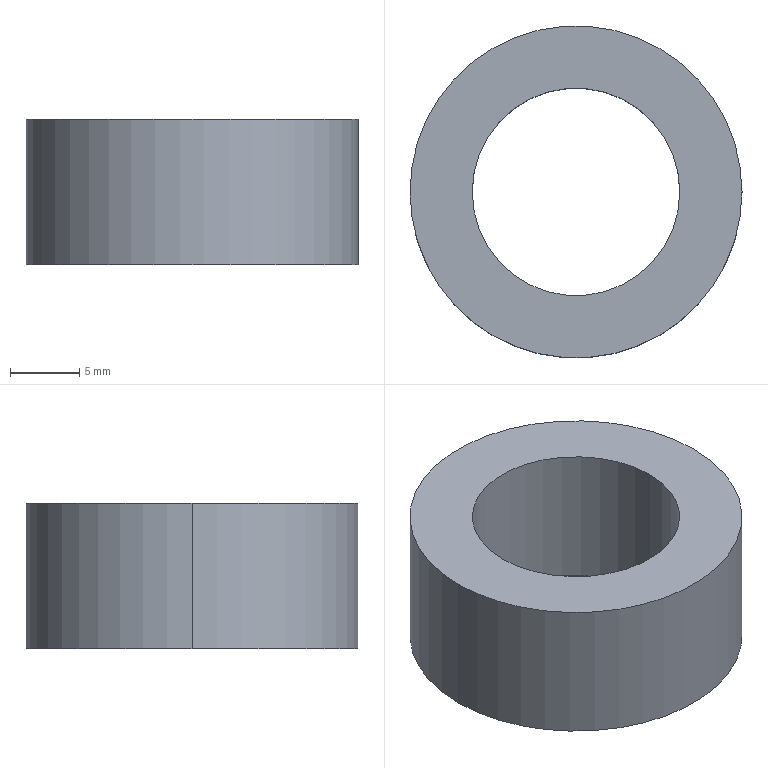Part | STEP file | PN_0019 (stop plate) | 1 solid | 6 faces | box 24 x 24 x 10.5 mm | volume 2895 mm3 | cylinder 4 | plane 2 | commonest cylinder face diameters 15 x2 24 x2
STEP:
#1=CARTESIAN_POINT('',(0.,0.,0.));
#2=DIRECTION('',(0.,0.,1.));
#3=DIRECTION('',(1.,0.,0.));
#4=AXIS2_PLACEMENT_3D('',#1,#2,#3);
#5=CARTESIAN_POINT('',(-7.5,0.,10.5));
#6=VERTEX_POINT('',#5);
#7=CARTESIAN_POINT('',(-7.5,0.,0.));
#8=VERTEX_POINT('',#7);
#9=CARTESIAN_POINT('',(-7.5,0.,10.5));
#10=DIRECTION('',(0.,0.,-1.));
#11=VECTOR('',#10,1.);
#12=LINE('',#9,#11);
#13=CARTESIAN_POINT('',(0.,0.,10.5));
#14=DIRECTION('',(0.,0.,-1.));
#15=DIRECTION('',(-1.,0.,0.));
#16=AXIS2_PLACEMENT_3D('',#13,#14,#15);
#17=CYLINDRICAL_SURFACE('',#16,7.5);
#18=CARTESIAN_POINT('',(6.283,0.));
#19=DIRECTION('',(0.,1.));
#20=VECTOR('',#19,1.);
#21=LINE('',#18,#20);
#22=(GEOMETRIC_REPRESENTATION_CONTEXT(2)PARAMETRIC_REPRESENTATION_CONTEXT()REPRESENTATION_CONTEXT('',''));
#23=DEFINITIONAL_REPRESENTATION('',(#21),#22);
#24=PCURVE('',#17,#23);
#25=CARTESIAN_POINT('',(0.,0.,10.5));
#26=DIRECTION('',(0.,0.,-1.));
#27=DIRECTION('',(-1.,0.,0.));
#28=AXIS2_PLACEMENT_3D('',#25,#26,#27);
#29=CYLINDRICAL_SURFACE('',#28,7.5);
#30=CARTESIAN_POINT('',(0.,0.));
#31=DIRECTION('',(0.,1.));
#32=VECTOR('',#31,1.);
#33=LINE('',#30,#32);
#34=(GEOMETRIC_REPRESENTATION_CONTEXT(2)PARAMETRIC_REPRESENTATION_CONTEXT()REPRESENTATION_CONTEXT('',''));
#35=DEFINITIONAL_REPRESENTATION('',(#33),#34);
#36=PCURVE('',#29,#35);
#37=SURFACE_CURVE('',#12,(#24,#36),.PCURVE_S1.);
#38=EDGE_CURVE('',#6,#8,#37,.T.);
#39=ORIENTED_EDGE('',*,*,#38,.T.);
#40=CARTESIAN_POINT('',(7.5,0.,0.));
#41=VERTEX_POINT('',#40);
#42=CARTESIAN_POINT('',(0.,0.,0.));
#43=DIRECTION('',(0.,0.,1.));
#44=DIRECTION('',(1.,0.,0.));
#45=AXIS2_PLACEMENT_3D('',#42,#43,#44);
#46=CIRCLE('',#45,7.5);
#47=CARTESIAN_POINT('',(9.425,10.5));
#48=DIRECTION('',(-1.,0.));
#49=VECTOR('',#48,1.);
#50=LINE('',#47,#49);
#51=(GEOMETRIC_REPRESENTATION_CONTEXT(2)PARAMETRIC_REPRESENTATION_CONTEXT()REPRESENTATION_CONTEXT('',''));
#52=DEFINITIONAL_REPRESENTATION('',(#50),#51);
#53=PCURVE('',#17,#52);
#54=CARTESIAN_POINT('',(0.,0.,0.));
#55=DIRECTION('',(0.,0.,1.));
#56=DIRECTION('',(1.,0.,0.));
#57=AXIS2_PLACEMENT_3D('',#54,#55,#56);
#58=PLANE('',#57);
#59=CARTESIAN_POINT('',(0.,0.));
#60=DIRECTION('',(1.,0.));
#61=AXIS2_PLACEMENT_2D('',#59,#60);
#62=CIRCLE('',#61,7.5);
#63=(GEOMETRIC_REPRESENTATION_CONTEXT(2)PARAMETRIC_REPRESENTATION_CONTEXT()REPRESENTATION_CONTEXT('',''));
#64=DEFINITIONAL_REPRESENTATION('',(#62),#63);
#65=PCURVE('',#58,#64);
#66=SURFACE_CURVE('',#46,(#53,#65),.PCURVE_S1.);
#67=EDGE_CURVE('',#8,#41,#66,.T.);
#68=ORIENTED_EDGE('',*,*,#67,.T.);
#69=CARTESIAN_POINT('',(7.5,0.,10.5));
#70=VERTEX_POINT('',#69);
#71=CARTESIAN_POINT('',(7.5,0.,10.5));
#72=DIRECTION('',(0.,0.,-1.));
#73=VECTOR('',#72,1.);
#74=LINE('',#71,#73);
#75=CARTESIAN_POINT('',(3.142,0.));
#76=DIRECTION('',(0.,1.));
#77=VECTOR('',#76,1.);
#78=LINE('',#75,#77);
#79=(GEOMETRIC_REPRESENTATION_CONTEXT(2)PARAMETRIC_REPRESENTATION_CONTEXT()REPRESENTATION_CONTEXT('',''));
#80=DEFINITIONAL_REPRESENTATION('',(#78),#79);
#81=PCURVE('',#17,#80);
#82=CARTESIAN_POINT('',(3.142,0.));
#83=DIRECTION('',(0.,1.));
#84=VECTOR('',#83,1.);
#85=LINE('',#82,#84);
#86=(GEOMETRIC_REPRESENTATION_CONTEXT(2)PARAMETRIC_REPRESENTATION_CONTEXT()REPRESENTATION_CONTEXT('',''));
#87=DEFINITIONAL_REPRESENTATION('',(#85),#86);
#88=PCURVE('',#29,#87);
#89=SURFACE_CURVE('',#74,(#81,#88),.PCURVE_S1.);
#90=EDGE_CURVE('',#70,#41,#89,.T.);
#91=ORIENTED_EDGE('',*,*,#90,.F.);
#92=CARTESIAN_POINT('',(0.,0.,10.5));
#93=DIRECTION('',(0.,0.,1.));
#94=DIRECTION('',(1.,0.,0.));
#95=AXIS2_PLACEMENT_3D('',#92,#93,#94);
#96=CIRCLE('',#95,7.5);
#97=CARTESIAN_POINT('',(9.425,0.));
#98=DIRECTION('',(-1.,0.));
#99=VECTOR('',#98,1.);
#100=LINE('',#97,#99);
#101=(GEOMETRIC_REPRESENTATION_CONTEXT(2)PARAMETRIC_REPRESENTATION_CONTEXT()REPRESENTATION_CONTEXT('',''));
#102=DEFINITIONAL_REPRESENTATION('',(#100),#101);
#103=PCURVE('',#17,#102);
#104=CARTESIAN_POINT('',(0.,0.,10.5));
#105=DIRECTION('',(0.,0.,1.));
#106=DIRECTION('',(1.,0.,0.));
#107=AXIS2_PLACEMENT_3D('',#104,#105,#106);
#108=PLANE('',#107);
#109=CARTESIAN_POINT('',(0.,0.));
#110=DIRECTION('',(1.,0.));
#111=AXIS2_PLACEMENT_2D('',#109,#110);
#112=CIRCLE('',#111,7.5);
#113=(GEOMETRIC_REPRESENTATION_CONTEXT(2)PARAMETRIC_REPRESENTATION_CONTEXT()REPRESENTATION_CONTEXT('',''));
#114=DEFINITIONAL_REPRESENTATION('',(#112),#113);
#115=PCURVE('',#108,#114);
#116=SURFACE_CURVE('',#96,(#103,#115),.PCURVE_S1.);
#117=EDGE_CURVE('',#6,#70,#116,.T.);
#118=ORIENTED_EDGE('',*,*,#117,.F.);
#119=EDGE_LOOP('',(#39,#68,#91,#118));
#120=FACE_BOUND('',#119,.F.);
#121=ADVANCED_FACE('',(#120),#17,.F.);
#122=CARTESIAN_POINT('',(12.,0.,10.5));
#123=VERTEX_POINT('',#122);
#124=CARTESIAN_POINT('',(-12.,0.,10.5));
#125=VERTEX_POINT('',#124);
#126=CARTESIAN_POINT('',(0.,0.,10.5));
#127=DIRECTION('',(0.,0.,1.));
#128=DIRECTION('',(1.,0.,0.));
#129=AXIS2_PLACEMENT_3D('',#126,#127,#128);
#130=CIRCLE('',#129,12.);
#131=CARTESIAN_POINT('',(0.,0.,10.5));
#132=DIRECTION('',(0.,0.,-1.));
#133=DIRECTION('',(-1.,0.,0.));
#134=AXIS2_PLACEMENT_3D('',#131,#132,#133);
#135=CYLINDRICAL_SURFACE('',#134,12.);
#136=CARTESIAN_POINT('',(3.142,0.));
#137=DIRECTION('',(-1.,0.));
#138=VECTOR('',#137,1.);
#139=LINE('',#136,#138);
#140=(GEOMETRIC_REPRESENTATION_CONTEXT(2)PARAMETRIC_REPRESENTATION_CONTEXT()REPRESENTATION_CONTEXT('',''));
#141=DEFINITIONAL_REPRESENTATION('',(#139),#140);
#142=PCURVE('',#135,#141);
#143=CARTESIAN_POINT('',(0.,0.));
#144=DIRECTION('',(1.,0.));
#145=AXIS2_PLACEMENT_2D('',#143,#144);
#146=CIRCLE('',#145,12.);
#147=(GEOMETRIC_REPRESENTATION_CONTEXT(2)PARAMETRIC_REPRESENTATION_CONTEXT()REPRESENTATION_CONTEXT('',''));
#148=DEFINITIONAL_REPRESENTATION('',(#146),#147);
#149=PCURVE('',#108,#148);
#150=SURFACE_CURVE('',#130,(#142,#149),.PCURVE_S1.);
#151=EDGE_CURVE('',#123,#125,#150,.T.);
#152=ORIENTED_EDGE('',*,*,#151,.F.);
#153=CARTESIAN_POINT('',(12.,0.,0.));
#154=VERTEX_POINT('',#153);
#155=CARTESIAN_POINT('',(12.,0.,10.5));
#156=DIRECTION('',(0.,0.,-1.));
#157=VECTOR('',#156,1.);
#158=LINE('',#155,#157);
#159=CARTESIAN_POINT('',(3.142,0.));
#160=DIRECTION('',(0.,1.));
#161=VECTOR('',#160,1.);
#162=LINE('',#159,#161);
#163=(GEOMETRIC_REPRESENTATION_CONTEXT(2)PARAMETRIC_REPRESENTATION_CONTEXT()REPRESENTATION_CONTEXT('',''));
#164=DEFINITIONAL_REPRESENTATION('',(#162),#163);
#165=PCURVE('',#135,#164);
#166=CARTESIAN_POINT('',(0.,0.,10.5));
#167=DIRECTION('',(0.,0.,-1.));
#168=DIRECTION('',(-1.,0.,0.));
#169=AXIS2_PLACEMENT_3D('',#166,#167,#168);
#170=CYLINDRICAL_SURFACE('',#169,12.);
#171=CARTESIAN_POINT('',(3.142,0.));
#172=DIRECTION('',(0.,1.));
#173=VECTOR('',#172,1.);
#174=LINE('',#171,#173);
#175=(GEOMETRIC_REPRESENTATION_CONTEXT(2)PARAMETRIC_REPRESENTATION_CONTEXT()REPRESENTATION_CONTEXT('',''));
#176=DEFINITIONAL_REPRESENTATION('',(#174),#175);
#177=PCURVE('',#170,#176);
#178=SURFACE_CURVE('',#158,(#165,#177),.PCURVE_S1.);
#179=EDGE_CURVE('',#123,#154,#178,.T.);
#180=ORIENTED_EDGE('',*,*,#179,.T.);
#181=CARTESIAN_POINT('',(-12.,0.,0.));
#182=VERTEX_POINT('',#181);
#183=CARTESIAN_POINT('',(0.,0.,0.));
#184=DIRECTION('',(0.,0.,1.));
#185=DIRECTION('',(1.,0.,0.));
#186=AXIS2_PLACEMENT_3D('',#183,#184,#185);
#187=CIRCLE('',#186,12.);
#188=CARTESIAN_POINT('',(3.142,10.5));
#189=DIRECTION('',(-1.,0.));
#190=VECTOR('',#189,1.);
#191=LINE('',#188,#190);
#192=(GEOMETRIC_REPRESENTATION_CONTEXT(2)PARAMETRIC_REPRESENTATION_CONTEXT()REPRESENTATION_CONTEXT('',''));
#193=DEFINITIONAL_REPRESENTATION('',(#191),#192);
#194=PCURVE('',#135,#193);
#195=CARTESIAN_POINT('',(0.,0.));
#196=DIRECTION('',(1.,0.));
#197=AXIS2_PLACEMENT_2D('',#195,#196);
#198=CIRCLE('',#197,12.);
#199=(GEOMETRIC_REPRESENTATION_CONTEXT(2)PARAMETRIC_REPRESENTATION_CONTEXT()REPRESENTATION_CONTEXT('',''));
#200=DEFINITIONAL_REPRESENTATION('',(#198),#199);
#201=PCURVE('',#58,#200);
#202=SURFACE_CURVE('',#187,(#194,#201),.PCURVE_S1.);
#203=EDGE_CURVE('',#154,#182,#202,.T.);
#204=ORIENTED_EDGE('',*,*,#203,.T.);
#205=CARTESIAN_POINT('',(-12.,0.,10.5));
#206=DIRECTION('',(0.,0.,-1.));
#207=VECTOR('',#206,1.);
#208=LINE('',#205,#207);
#209=CARTESIAN_POINT('',(0.,0.));
#210=DIRECTION('',(0.,1.));
#211=VECTOR('',#210,1.);
#212=LINE('',#209,#211);
#213=(GEOMETRIC_REPRESENTATION_CONTEXT(2)PARAMETRIC_REPRESENTATION_CONTEXT()REPRESENTATION_CONTEXT('',''));
#214=DEFINITIONAL_REPRESENTATION('',(#212),#213);
#215=PCURVE('',#135,#214);
#216=CARTESIAN_POINT('',(6.283,0.));
#217=DIRECTION('',(0.,1.));
#218=VECTOR('',#217,1.);
#219=LINE('',#216,#218);
#220=(GEOMETRIC_REPRESENTATION_CONTEXT(2)PARAMETRIC_REPRESENTATION_CONTEXT()REPRESENTATION_CONTEXT('',''));
#221=DEFINITIONAL_REPRESENTATION('',(#219),#220);
#222=PCURVE('',#170,#221);
#223=SURFACE_CURVE('',#208,(#215,#222),.PCURVE_S1.);
#224=EDGE_CURVE('',#125,#182,#223,.T.);
#225=ORIENTED_EDGE('',*,*,#224,.F.);
#226=EDGE_LOOP('',(#152,#180,#204,#225));
#227=FACE_BOUND('',#226,.T.);
#228=ADVANCED_FACE('',(#227),#135,.T.);
#229=CARTESIAN_POINT('',(0.,0.,10.5));
#230=DIRECTION('',(0.,0.,1.));
#231=DIRECTION('',(1.,0.,0.));
#232=AXIS2_PLACEMENT_3D('',#229,#230,#231);
#233=CIRCLE('',#232,12.);
#234=CARTESIAN_POINT('',(0.,0.));
#235=DIRECTION('',(1.,0.));
#236=AXIS2_PLACEMENT_2D('',#234,#235);
#237=CIRCLE('',#236,12.);
#238=(GEOMETRIC_REPRESENTATION_CONTEXT(2)PARAMETRIC_REPRESENTATION_CONTEXT()REPRESENTATION_CONTEXT('',''));
#239=DEFINITIONAL_REPRESENTATION('',(#237),#238);
#240=PCURVE('',#108,#239);
#241=CARTESIAN_POINT('',(9.425,0.));
#242=DIRECTION('',(-1.,0.));
#243=VECTOR('',#242,1.);
#244=LINE('',#241,#243);
#245=(GEOMETRIC_REPRESENTATION_CONTEXT(2)PARAMETRIC_REPRESENTATION_CONTEXT()REPRESENTATION_CONTEXT('',''));
#246=DEFINITIONAL_REPRESENTATION('',(#244),#245);
#247=PCURVE('',#170,#246);
#248=SURFACE_CURVE('',#233,(#240,#247),.PCURVE_S1.);
#249=EDGE_CURVE('',#125,#123,#248,.T.);
#250=ORIENTED_EDGE('',*,*,#249,.T.);
#251=ORIENTED_EDGE('',*,*,#151,.T.);
#252=EDGE_LOOP('',(#250,#251));
#253=FACE_BOUND('',#252,.T.);
#254=ORIENTED_EDGE('',*,*,#117,.F.);
#255=CARTESIAN_POINT('',(0.,0.,10.5));
#256=DIRECTION('',(0.,0.,1.));
#257=DIRECTION('',(1.,0.,0.));
#258=AXIS2_PLACEMENT_3D('',#255,#256,#257);
#259=CIRCLE('',#258,7.5);
#260=CARTESIAN_POINT('',(0.,0.));
#261=DIRECTION('',(1.,0.));
#262=AXIS2_PLACEMENT_2D('',#260,#261);
#263=CIRCLE('',#262,7.5);
#264=(GEOMETRIC_REPRESENTATION_CONTEXT(2)PARAMETRIC_REPRESENTATION_CONTEXT()REPRESENTATION_CONTEXT('',''));
#265=DEFINITIONAL_REPRESENTATION('',(#263),#264);
#266=PCURVE('',#108,#265);
#267=CARTESIAN_POINT('',(3.142,0.));
#268=DIRECTION('',(-1.,0.));
#269=VECTOR('',#268,1.);
#270=LINE('',#267,#269);
#271=(GEOMETRIC_REPRESENTATION_CONTEXT(2)PARAMETRIC_REPRESENTATION_CONTEXT()REPRESENTATION_CONTEXT('',''));
#272=DEFINITIONAL_REPRESENTATION('',(#270),#271);
#273=PCURVE('',#29,#272);
#274=SURFACE_CURVE('',#259,(#266,#273),.PCURVE_S1.);
#275=EDGE_CURVE('',#70,#6,#274,.T.);
#276=ORIENTED_EDGE('',*,*,#275,.F.);
#277=EDGE_LOOP('',(#254,#276));
#278=FACE_BOUND('',#277,.T.);
#279=ADVANCED_FACE('',(#253,#278),#108,.T.);
#280=CARTESIAN_POINT('',(0.,0.,0.));
#281=DIRECTION('',(0.,0.,1.));
#282=DIRECTION('',(1.,0.,0.));
#283=AXIS2_PLACEMENT_3D('',#280,#281,#282);
#284=CIRCLE('',#283,12.);
#285=CARTESIAN_POINT('',(0.,0.));
#286=DIRECTION('',(1.,0.));
#287=AXIS2_PLACEMENT_2D('',#285,#286);
#288=CIRCLE('',#287,12.);
#289=(GEOMETRIC_REPRESENTATION_CONTEXT(2)PARAMETRIC_REPRESENTATION_CONTEXT()REPRESENTATION_CONTEXT('',''));
#290=DEFINITIONAL_REPRESENTATION('',(#288),#289);
#291=PCURVE('',#58,#290);
#292=CARTESIAN_POINT('',(9.425,10.5));
#293=DIRECTION('',(-1.,0.));
#294=VECTOR('',#293,1.);
#295=LINE('',#292,#294);
#296=(GEOMETRIC_REPRESENTATION_CONTEXT(2)PARAMETRIC_REPRESENTATION_CONTEXT()REPRESENTATION_CONTEXT('',''));
#297=DEFINITIONAL_REPRESENTATION('',(#295),#296);
#298=PCURVE('',#170,#297);
#299=SURFACE_CURVE('',#284,(#291,#298),.PCURVE_S1.);
#300=EDGE_CURVE('',#182,#154,#299,.T.);
#301=ORIENTED_EDGE('',*,*,#300,.F.);
#302=ORIENTED_EDGE('',*,*,#203,.F.);
#303=EDGE_LOOP('',(#301,#302));
#304=FACE_BOUND('',#303,.T.);
#305=ORIENTED_EDGE('',*,*,#67,.T.);
#306=CARTESIAN_POINT('',(0.,0.,0.));
#307=DIRECTION('',(0.,0.,1.));
#308=DIRECTION('',(1.,0.,0.));
#309=AXIS2_PLACEMENT_3D('',#306,#307,#308);
#310=CIRCLE('',#309,7.5);
#311=CARTESIAN_POINT('',(0.,0.));
#312=DIRECTION('',(1.,0.));
#313=AXIS2_PLACEMENT_2D('',#311,#312);
#314=CIRCLE('',#313,7.5);
#315=(GEOMETRIC_REPRESENTATION_CONTEXT(2)PARAMETRIC_REPRESENTATION_CONTEXT()REPRESENTATION_CONTEXT('',''));
#316=DEFINITIONAL_REPRESENTATION('',(#314),#315);
#317=PCURVE('',#58,#316);
#318=CARTESIAN_POINT('',(3.142,10.5));
#319=DIRECTION('',(-1.,0.));
#320=VECTOR('',#319,1.);
#321=LINE('',#318,#320);
#322=(GEOMETRIC_REPRESENTATION_CONTEXT(2)PARAMETRIC_REPRESENTATION_CONTEXT()REPRESENTATION_CONTEXT('',''));
#323=DEFINITIONAL_REPRESENTATION('',(#321),#322);
#324=PCURVE('',#29,#323);
#325=SURFACE_CURVE('',#310,(#317,#324),.PCURVE_S1.);
#326=EDGE_CURVE('',#41,#8,#325,.T.);
#327=ORIENTED_EDGE('',*,*,#326,.T.);
#328=EDGE_LOOP('',(#305,#327));
#329=FACE_BOUND('',#328,.T.);
#330=ADVANCED_FACE('',(#304,#329),#58,.F.);
#331=ORIENTED_EDGE('',*,*,#179,.F.);
#332=ORIENTED_EDGE('',*,*,#249,.F.);
#333=ORIENTED_EDGE('',*,*,#224,.T.);
#334=ORIENTED_EDGE('',*,*,#300,.T.);
#335=EDGE_LOOP('',(#331,#332,#333,#334));
#336=FACE_BOUND('',#335,.T.);
#337=ADVANCED_FACE('',(#336),#170,.T.);
#338=ORIENTED_EDGE('',*,*,#326,.T.);
#339=ORIENTED_EDGE('',*,*,#38,.F.);
#340=ORIENTED_EDGE('',*,*,#275,.F.);
#341=ORIENTED_EDGE('',*,*,#90,.T.);
#342=EDGE_LOOP('',(#338,#339,#340,#341));
#343=FACE_BOUND('',#342,.F.);
#344=ADVANCED_FACE('',(#343),#29,.F.);
#345=CLOSED_SHELL('',(#121,#228,#279,#330,#337,#344));
#346=MANIFOLD_SOLID_BREP('',#345);
#347=(LENGTH_UNIT()NAMED_UNIT(*)SI_UNIT(.MILLI.,.METRE.));
#348=UNCERTAINTY_MEASURE_WITH_UNIT(LENGTH_MEASURE(0.0000001),#347,'','');
#349=(NAMED_UNIT(*)PLANE_ANGLE_UNIT()SI_UNIT($,.RADIAN.));
#350=(NAMED_UNIT(*)SI_UNIT($,.STERADIAN.)SOLID_ANGLE_UNIT());
#351=(GEOMETRIC_REPRESENTATION_CONTEXT(3)GLOBAL_UNCERTAINTY_ASSIGNED_CONTEXT((#348))GLOBAL_UNIT_ASSIGNED_CONTEXT((#347,#349,#350))REPRESENTATION_CONTEXT('',''));
#352=ADVANCED_BREP_SHAPE_REPRESENTATION('',(#4,#346),#351);